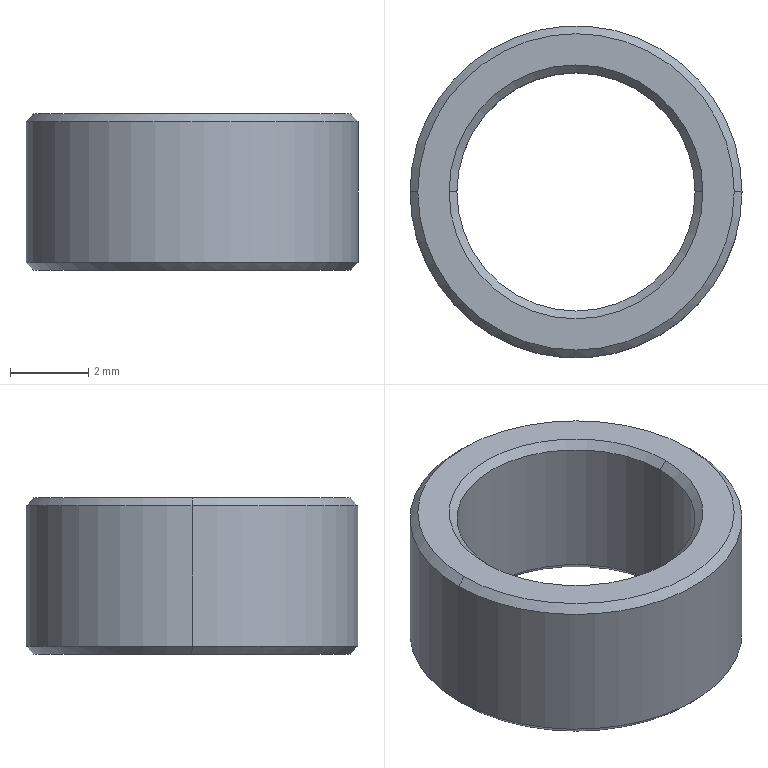Part | NX | features BREP 1 | 1 solid | 14 faces | box 8.5 x 8.5 x 4 mm | volume 108.247 mm3 | cone 8 | cylinder 4 | plane 2 | commonest cylinder face diameters 6.1 x2 8.5 x2
STEP:
#1=CARTESIAN_POINT('',(-3.25,0.,4.));
#2=VERTEX_POINT('',#1);
#3=CARTESIAN_POINT('',(-3.05,0.,3.8));
#4=VERTEX_POINT('',#3);
#5=CARTESIAN_POINT('',(-3.05,0.,3.8));
#6=DIRECTION('',(-0.7071,0.,0.7071));
#7=VECTOR('',#6,1000.);
#8=LINE('',#5,#7);
#9=EDGE_CURVE('',#2,#4,#8,.F.);
#10=ORIENTED_EDGE('',*,*,#9,.T.);
#11=CARTESIAN_POINT('',(3.05,0.,3.8));
#12=VERTEX_POINT('',#11);
#13=CARTESIAN_POINT('',(0.,0.,3.8));
#14=DIRECTION('',(0.,0.,1.));
#15=DIRECTION('',(1.,0.,0.));
#16=AXIS2_PLACEMENT_3D('',#13,#14,#15);
#17=CIRCLE('',#16,3.05);
#18=EDGE_CURVE('',#12,#4,#17,.T.);
#19=ORIENTED_EDGE('',*,*,#18,.F.);
#20=CARTESIAN_POINT('',(3.25,0.,4.));
#21=VERTEX_POINT('',#20);
#22=CARTESIAN_POINT('',(3.05,0.,3.8));
#23=DIRECTION('',(0.7071,0.,0.7071));
#24=VECTOR('',#23,1000.);
#25=LINE('',#22,#24);
#26=EDGE_CURVE('',#21,#12,#25,.F.);
#27=ORIENTED_EDGE('',*,*,#26,.F.);
#28=CARTESIAN_POINT('',(0.,0.,4.));
#29=DIRECTION('',(0.,0.,-1.));
#30=DIRECTION('',(1.,0.,0.));
#31=AXIS2_PLACEMENT_3D('',#28,#29,#30);
#32=CIRCLE('',#31,3.25);
#33=EDGE_CURVE('',#2,#21,#32,.T.);
#34=ORIENTED_EDGE('',*,*,#33,.F.);
#35=EDGE_LOOP('',(#10,#19,#27,#34));
#36=FACE_BOUND('',#35,.T.);
#37=CARTESIAN_POINT('',(0.,0.,3.8));
#38=DIRECTION('',(0.,0.,1.));
#39=DIRECTION('',(1.,0.,0.));
#40=AXIS2_PLACEMENT_3D('',#37,#38,#39);
#41=CONICAL_SURFACE('',#40,3.05,0.7854);
#42=ADVANCED_FACE('',(#36),#41,.F.);
#43=CARTESIAN_POINT('',(4.05,0.,4.));
#44=VERTEX_POINT('',#43);
#45=CARTESIAN_POINT('',(4.25,0.,3.8));
#46=VERTEX_POINT('',#45);
#47=CARTESIAN_POINT('',(4.05,0.,4.));
#48=DIRECTION('',(0.7071,0.,-0.7071));
#49=VECTOR('',#48,1000.);
#50=LINE('',#47,#49);
#51=EDGE_CURVE('',#44,#46,#50,.T.);
#52=ORIENTED_EDGE('',*,*,#51,.F.);
#53=CARTESIAN_POINT('',(-4.05,0.,4.));
#54=VERTEX_POINT('',#53);
#55=CARTESIAN_POINT('',(0.,0.,4.));
#56=DIRECTION('',(0.,0.,1.));
#57=DIRECTION('',(1.,0.,0.));
#58=AXIS2_PLACEMENT_3D('',#55,#56,#57);
#59=CIRCLE('',#58,4.05);
#60=EDGE_CURVE('',#54,#44,#59,.T.);
#61=ORIENTED_EDGE('',*,*,#60,.F.);
#62=CARTESIAN_POINT('',(-4.25,0.,3.8));
#63=VERTEX_POINT('',#62);
#64=CARTESIAN_POINT('',(-4.05,0.,4.));
#65=DIRECTION('',(-0.7071,0.,-0.7071));
#66=VECTOR('',#65,1000.);
#67=LINE('',#64,#66);
#68=EDGE_CURVE('',#54,#63,#67,.T.);
#69=ORIENTED_EDGE('',*,*,#68,.T.);
#70=CARTESIAN_POINT('',(0.,0.,3.8));
#71=DIRECTION('',(0.,0.,-1.));
#72=DIRECTION('',(1.,0.,0.));
#73=AXIS2_PLACEMENT_3D('',#70,#71,#72);
#74=CIRCLE('',#73,4.25);
#75=EDGE_CURVE('',#46,#63,#74,.T.);
#76=ORIENTED_EDGE('',*,*,#75,.F.);
#77=EDGE_LOOP('',(#52,#61,#69,#76));
#78=FACE_BOUND('',#77,.T.);
#79=CARTESIAN_POINT('',(0.,0.,4.));
#80=DIRECTION('',(0.,0.,-1.));
#81=DIRECTION('',(-1.,0.,0.));
#82=AXIS2_PLACEMENT_3D('',#79,#80,#81);
#83=CONICAL_SURFACE('',#82,4.05,0.7854);
#84=ADVANCED_FACE('',(#78),#83,.T.);
#85=CARTESIAN_POINT('',(-4.25,0.,0.2));
#86=VERTEX_POINT('',#85);
#87=CARTESIAN_POINT('',(-4.05,0.,0.));
#88=VERTEX_POINT('',#87);
#89=CARTESIAN_POINT('',(-4.25,0.,0.2));
#90=DIRECTION('',(-0.7071,0.,0.7071));
#91=VECTOR('',#90,1000.);
#92=LINE('',#89,#91);
#93=EDGE_CURVE('',#86,#88,#92,.F.);
#94=ORIENTED_EDGE('',*,*,#93,.T.);
#95=CARTESIAN_POINT('',(4.05,0.,0.));
#96=VERTEX_POINT('',#95);
#97=CARTESIAN_POINT('',(0.,0.,0.));
#98=DIRECTION('',(0.,0.,-1.));
#99=DIRECTION('',(1.,0.,0.));
#100=AXIS2_PLACEMENT_3D('',#97,#98,#99);
#101=CIRCLE('',#100,4.05);
#102=EDGE_CURVE('',#96,#88,#101,.T.);
#103=ORIENTED_EDGE('',*,*,#102,.F.);
#104=CARTESIAN_POINT('',(4.25,0.,0.2));
#105=VERTEX_POINT('',#104);
#106=CARTESIAN_POINT('',(4.25,0.,0.2));
#107=DIRECTION('',(0.7071,0.,0.7071));
#108=VECTOR('',#107,1000.);
#109=LINE('',#106,#108);
#110=EDGE_CURVE('',#105,#96,#109,.F.);
#111=ORIENTED_EDGE('',*,*,#110,.F.);
#112=CARTESIAN_POINT('',(0.,0.,0.2));
#113=DIRECTION('',(0.,0.,1.));
#114=DIRECTION('',(1.,0.,0.));
#115=AXIS2_PLACEMENT_3D('',#112,#113,#114);
#116=CIRCLE('',#115,4.25);
#117=EDGE_CURVE('',#86,#105,#116,.T.);
#118=ORIENTED_EDGE('',*,*,#117,.F.);
#119=EDGE_LOOP('',(#94,#103,#111,#118));
#120=FACE_BOUND('',#119,.T.);
#121=CARTESIAN_POINT('',(0.,0.,0.2));
#122=DIRECTION('',(0.,0.,1.));
#123=DIRECTION('',(1.,0.,0.));
#124=AXIS2_PLACEMENT_3D('',#121,#122,#123);
#125=CONICAL_SURFACE('',#124,4.25,0.7854);
#126=ADVANCED_FACE('',(#120),#125,.T.);
#127=CARTESIAN_POINT('',(3.05,0.,0.2));
#128=VERTEX_POINT('',#127);
#129=CARTESIAN_POINT('',(3.25,0.,0.));
#130=VERTEX_POINT('',#129);
#131=CARTESIAN_POINT('',(3.25,0.,0.));
#132=DIRECTION('',(0.7071,0.,-0.7071));
#133=VECTOR('',#132,1000.);
#134=LINE('',#131,#133);
#135=EDGE_CURVE('',#128,#130,#134,.T.);
#136=ORIENTED_EDGE('',*,*,#135,.F.);
#137=CARTESIAN_POINT('',(-3.05,0.,0.2));
#138=VERTEX_POINT('',#137);
#139=CARTESIAN_POINT('',(0.,0.,0.2));
#140=DIRECTION('',(0.,0.,-1.));
#141=DIRECTION('',(1.,0.,0.));
#142=AXIS2_PLACEMENT_3D('',#139,#140,#141);
#143=CIRCLE('',#142,3.05);
#144=EDGE_CURVE('',#138,#128,#143,.T.);
#145=ORIENTED_EDGE('',*,*,#144,.F.);
#146=CARTESIAN_POINT('',(-3.25,0.,0.));
#147=VERTEX_POINT('',#146);
#148=CARTESIAN_POINT('',(-3.25,0.,0.));
#149=DIRECTION('',(-0.7071,0.,-0.7071));
#150=VECTOR('',#149,1000.);
#151=LINE('',#148,#150);
#152=EDGE_CURVE('',#138,#147,#151,.T.);
#153=ORIENTED_EDGE('',*,*,#152,.T.);
#154=CARTESIAN_POINT('',(0.,0.,0.));
#155=DIRECTION('',(0.,0.,1.));
#156=DIRECTION('',(1.,0.,0.));
#157=AXIS2_PLACEMENT_3D('',#154,#155,#156);
#158=CIRCLE('',#157,3.25);
#159=EDGE_CURVE('',#130,#147,#158,.T.);
#160=ORIENTED_EDGE('',*,*,#159,.F.);
#161=EDGE_LOOP('',(#136,#145,#153,#160));
#162=FACE_BOUND('',#161,.T.);
#163=CARTESIAN_POINT('',(0.,0.,0.));
#164=DIRECTION('',(0.,0.,-1.));
#165=DIRECTION('',(-1.,0.,0.));
#166=AXIS2_PLACEMENT_3D('',#163,#164,#165);
#167=CONICAL_SURFACE('',#166,3.25,0.7854);
#168=ADVANCED_FACE('',(#162),#167,.F.);
#169=CARTESIAN_POINT('',(3.05,0.,4.));
#170=DIRECTION('',(0.,0.,-1.));
#171=VECTOR('',#170,1000.);
#172=LINE('',#169,#171);
#173=EDGE_CURVE('',#12,#128,#172,.T.);
#174=ORIENTED_EDGE('',*,*,#173,.F.);
#175=ORIENTED_EDGE('',*,*,#18,.T.);
#176=CARTESIAN_POINT('',(-3.05,0.,4.));
#177=DIRECTION('',(0.,0.,-1.));
#178=VECTOR('',#177,1000.);
#179=LINE('',#176,#178);
#180=EDGE_CURVE('',#4,#138,#179,.T.);
#181=ORIENTED_EDGE('',*,*,#180,.T.);
#182=ORIENTED_EDGE('',*,*,#144,.T.);
#183=EDGE_LOOP('',(#174,#175,#181,#182));
#184=FACE_BOUND('',#183,.T.);
#185=CARTESIAN_POINT('',(0.,0.,4.));
#186=DIRECTION('',(0.,0.,-1.));
#187=DIRECTION('',(-1.,0.,0.));
#188=AXIS2_PLACEMENT_3D('',#185,#186,#187);
#189=CYLINDRICAL_SURFACE('',#188,3.05);
#190=ADVANCED_FACE('',(#184),#189,.F.);
#191=CARTESIAN_POINT('',(4.25,0.,4.));
#192=DIRECTION('',(0.,0.,-1.));
#193=VECTOR('',#192,1000.);
#194=LINE('',#191,#193);
#195=EDGE_CURVE('',#46,#105,#194,.T.);
#196=ORIENTED_EDGE('',*,*,#195,.F.);
#197=ORIENTED_EDGE('',*,*,#75,.T.);
#198=CARTESIAN_POINT('',(-4.25,0.,4.));
#199=DIRECTION('',(0.,0.,-1.));
#200=VECTOR('',#199,1000.);
#201=LINE('',#198,#200);
#202=EDGE_CURVE('',#63,#86,#201,.T.);
#203=ORIENTED_EDGE('',*,*,#202,.T.);
#204=ORIENTED_EDGE('',*,*,#117,.T.);
#205=EDGE_LOOP('',(#196,#197,#203,#204));
#206=FACE_BOUND('',#205,.T.);
#207=CARTESIAN_POINT('',(0.,0.,4.));
#208=DIRECTION('',(0.,0.,-1.));
#209=DIRECTION('',(-1.,0.,0.));
#210=AXIS2_PLACEMENT_3D('',#207,#208,#209);
#211=CYLINDRICAL_SURFACE('',#210,4.25);
#212=ADVANCED_FACE('',(#206),#211,.T.);
#213=ORIENTED_EDGE('',*,*,#102,.T.);
#214=CARTESIAN_POINT('',(0.,0.,0.));
#215=DIRECTION('',(0.,0.,-1.));
#216=DIRECTION('',(1.,0.,0.));
#217=AXIS2_PLACEMENT_3D('',#214,#215,#216);
#218=CIRCLE('',#217,4.05);
#219=EDGE_CURVE('',#88,#96,#218,.T.);
#220=ORIENTED_EDGE('',*,*,#219,.T.);
#221=EDGE_LOOP('',(#213,#220));
#222=FACE_BOUND('',#221,.T.);
#223=CARTESIAN_POINT('',(0.,0.,0.));
#224=DIRECTION('',(0.,0.,1.));
#225=DIRECTION('',(1.,0.,0.));
#226=AXIS2_PLACEMENT_3D('',#223,#224,#225);
#227=CIRCLE('',#226,3.25);
#228=EDGE_CURVE('',#147,#130,#227,.T.);
#229=ORIENTED_EDGE('',*,*,#228,.T.);
#230=ORIENTED_EDGE('',*,*,#159,.T.);
#231=EDGE_LOOP('',(#229,#230));
#232=FACE_BOUND('',#231,.T.);
#233=CARTESIAN_POINT('',(0.,0.,0.));
#234=DIRECTION('',(0.,0.,1.));
#235=DIRECTION('',(1.,0.,0.));
#236=AXIS2_PLACEMENT_3D('',#233,#234,#235);
#237=PLANE('',#236);
#238=ADVANCED_FACE('',(#222,#232),#237,.F.);
#239=CARTESIAN_POINT('',(0.,0.,4.));
#240=DIRECTION('',(0.,0.,-1.));
#241=DIRECTION('',(1.,0.,0.));
#242=AXIS2_PLACEMENT_3D('',#239,#240,#241);
#243=CIRCLE('',#242,3.25);
#244=EDGE_CURVE('',#21,#2,#243,.T.);
#245=ORIENTED_EDGE('',*,*,#244,.T.);
#246=ORIENTED_EDGE('',*,*,#33,.T.);
#247=EDGE_LOOP('',(#245,#246));
#248=FACE_BOUND('',#247,.T.);
#249=ORIENTED_EDGE('',*,*,#60,.T.);
#250=CARTESIAN_POINT('',(0.,0.,4.));
#251=DIRECTION('',(0.,0.,1.));
#252=DIRECTION('',(1.,0.,0.));
#253=AXIS2_PLACEMENT_3D('',#250,#251,#252);
#254=CIRCLE('',#253,4.05);
#255=EDGE_CURVE('',#44,#54,#254,.T.);
#256=ORIENTED_EDGE('',*,*,#255,.T.);
#257=EDGE_LOOP('',(#249,#256));
#258=FACE_BOUND('',#257,.T.);
#259=CARTESIAN_POINT('',(0.,0.,4.));
#260=DIRECTION('',(0.,0.,1.));
#261=DIRECTION('',(1.,0.,0.));
#262=AXIS2_PLACEMENT_3D('',#259,#260,#261);
#263=PLANE('',#262);
#264=ADVANCED_FACE('',(#248,#258),#263,.T.);
#265=CARTESIAN_POINT('',(0.,0.,3.8));
#266=DIRECTION('',(0.,0.,-1.));
#267=DIRECTION('',(1.,0.,0.));
#268=AXIS2_PLACEMENT_3D('',#265,#266,#267);
#269=CIRCLE('',#268,4.25);
#270=EDGE_CURVE('',#63,#46,#269,.T.);
#271=ORIENTED_EDGE('',*,*,#270,.T.);
#272=ORIENTED_EDGE('',*,*,#195,.T.);
#273=CARTESIAN_POINT('',(0.,0.,0.2));
#274=DIRECTION('',(0.,0.,1.));
#275=DIRECTION('',(1.,0.,0.));
#276=AXIS2_PLACEMENT_3D('',#273,#274,#275);
#277=CIRCLE('',#276,4.25);
#278=EDGE_CURVE('',#105,#86,#277,.T.);
#279=ORIENTED_EDGE('',*,*,#278,.T.);
#280=ORIENTED_EDGE('',*,*,#202,.F.);
#281=EDGE_LOOP('',(#271,#272,#279,#280));
#282=FACE_BOUND('',#281,.T.);
#283=CARTESIAN_POINT('',(0.,0.,4.));
#284=DIRECTION('',(0.,0.,-1.));
#285=DIRECTION('',(-1.,0.,0.));
#286=AXIS2_PLACEMENT_3D('',#283,#284,#285);
#287=CYLINDRICAL_SURFACE('',#286,4.25);
#288=ADVANCED_FACE('',(#282),#287,.T.);
#289=CARTESIAN_POINT('',(0.,0.,3.8));
#290=DIRECTION('',(0.,0.,1.));
#291=DIRECTION('',(1.,0.,0.));
#292=AXIS2_PLACEMENT_3D('',#289,#290,#291);
#293=CIRCLE('',#292,3.05);
#294=EDGE_CURVE('',#4,#12,#293,.T.);
#295=ORIENTED_EDGE('',*,*,#294,.T.);
#296=ORIENTED_EDGE('',*,*,#173,.T.);
#297=CARTESIAN_POINT('',(0.,0.,0.2));
#298=DIRECTION('',(0.,0.,-1.));
#299=DIRECTION('',(1.,0.,0.));
#300=AXIS2_PLACEMENT_3D('',#297,#298,#299);
#301=CIRCLE('',#300,3.05);
#302=EDGE_CURVE('',#128,#138,#301,.T.);
#303=ORIENTED_EDGE('',*,*,#302,.T.);
#304=ORIENTED_EDGE('',*,*,#180,.F.);
#305=EDGE_LOOP('',(#295,#296,#303,#304));
#306=FACE_BOUND('',#305,.T.);
#307=CARTESIAN_POINT('',(0.,0.,4.));
#308=DIRECTION('',(0.,0.,-1.));
#309=DIRECTION('',(-1.,0.,0.));
#310=AXIS2_PLACEMENT_3D('',#307,#308,#309);
#311=CYLINDRICAL_SURFACE('',#310,3.05);
#312=ADVANCED_FACE('',(#306),#311,.F.);
#313=ORIENTED_EDGE('',*,*,#302,.F.);
#314=ORIENTED_EDGE('',*,*,#135,.T.);
#315=ORIENTED_EDGE('',*,*,#228,.F.);
#316=ORIENTED_EDGE('',*,*,#152,.F.);
#317=EDGE_LOOP('',(#313,#314,#315,#316));
#318=FACE_BOUND('',#317,.T.);
#319=CARTESIAN_POINT('',(0.,0.,0.));
#320=DIRECTION('',(0.,0.,-1.));
#321=DIRECTION('',(-1.,0.,0.));
#322=AXIS2_PLACEMENT_3D('',#319,#320,#321);
#323=CONICAL_SURFACE('',#322,3.25,0.7854);
#324=ADVANCED_FACE('',(#318),#323,.F.);
#325=ORIENTED_EDGE('',*,*,#219,.F.);
#326=ORIENTED_EDGE('',*,*,#93,.F.);
#327=ORIENTED_EDGE('',*,*,#278,.F.);
#328=ORIENTED_EDGE('',*,*,#110,.T.);
#329=EDGE_LOOP('',(#325,#326,#327,#328));
#330=FACE_BOUND('',#329,.T.);
#331=CARTESIAN_POINT('',(0.,0.,0.2));
#332=DIRECTION('',(0.,0.,1.));
#333=DIRECTION('',(1.,0.,0.));
#334=AXIS2_PLACEMENT_3D('',#331,#332,#333);
#335=CONICAL_SURFACE('',#334,4.25,0.7854);
#336=ADVANCED_FACE('',(#330),#335,.T.);
#337=ORIENTED_EDGE('',*,*,#255,.F.);
#338=ORIENTED_EDGE('',*,*,#51,.T.);
#339=ORIENTED_EDGE('',*,*,#270,.F.);
#340=ORIENTED_EDGE('',*,*,#68,.F.);
#341=EDGE_LOOP('',(#337,#338,#339,#340));
#342=FACE_BOUND('',#341,.T.);
#343=CARTESIAN_POINT('',(0.,0.,4.));
#344=DIRECTION('',(0.,0.,-1.));
#345=DIRECTION('',(-1.,0.,0.));
#346=AXIS2_PLACEMENT_3D('',#343,#344,#345);
#347=CONICAL_SURFACE('',#346,4.05,0.7854);
#348=ADVANCED_FACE('',(#342),#347,.T.);
#349=ORIENTED_EDGE('',*,*,#294,.F.);
#350=ORIENTED_EDGE('',*,*,#9,.F.);
#351=ORIENTED_EDGE('',*,*,#244,.F.);
#352=ORIENTED_EDGE('',*,*,#26,.T.);
#353=EDGE_LOOP('',(#349,#350,#351,#352));
#354=FACE_BOUND('',#353,.T.);
#355=CARTESIAN_POINT('',(0.,0.,3.8));
#356=DIRECTION('',(0.,0.,1.));
#357=DIRECTION('',(1.,0.,0.));
#358=AXIS2_PLACEMENT_3D('',#355,#356,#357);
#359=CONICAL_SURFACE('',#358,3.05,0.7854);
#360=ADVANCED_FACE('',(#354),#359,.F.);
#361=CLOSED_SHELL('',(#42,#84,#126,#168,#190,#212,#238,#264,#288,#312,#324,#336,#348,#360));
#362=MANIFOLD_SOLID_BREP('',#361);
#363=(LENGTH_UNIT()NAMED_UNIT(*)SI_UNIT(.MILLI.,.METRE.));
#364=UNCERTAINTY_MEASURE_WITH_UNIT(LENGTH_MEASURE(0.00001),#363,'','');
#365=(NAMED_UNIT(*)PLANE_ANGLE_UNIT()SI_UNIT($,.RADIAN.));
#366=(NAMED_UNIT(*)SI_UNIT($,.STERADIAN.)SOLID_ANGLE_UNIT());
#367=(GEOMETRIC_REPRESENTATION_CONTEXT(3)GLOBAL_UNCERTAINTY_ASSIGNED_CONTEXT((#364))GLOBAL_UNIT_ASSIGNED_CONTEXT((#363,#365,#366))REPRESENTATION_CONTEXT('',''));
#368=ADVANCED_BREP_SHAPE_REPRESENTATION('',(#362),#367);